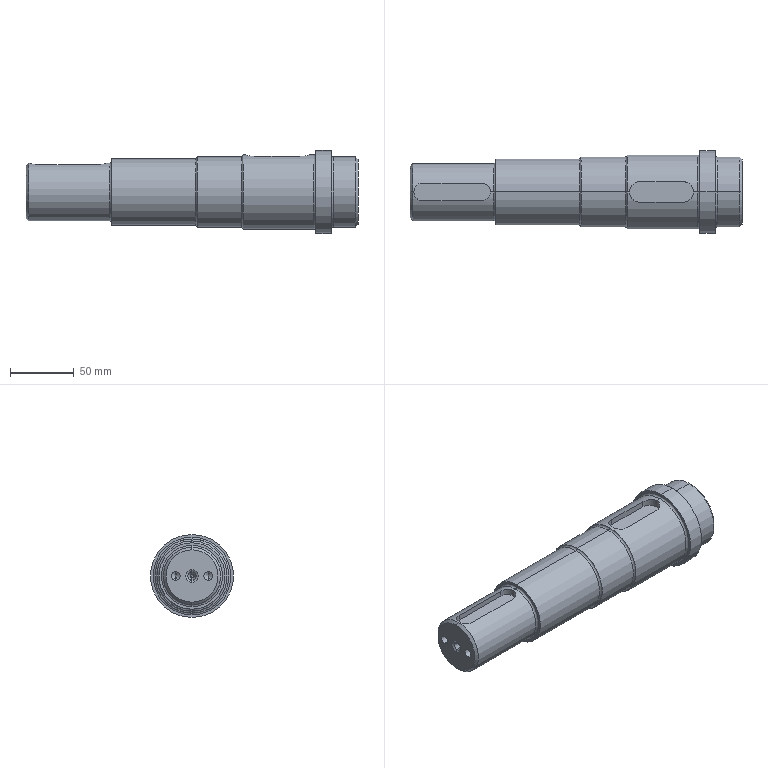Part | SolidWorks | features ICE 2, 3DProfileFeature 1, Chamfer 1, Fillet 1, HoleWzd 1, MirrorPattern 1, RevCut 1, Revolution 1 | 1 solid | 59 faces | box 260 x 65 x 65 mm | volume 565066 mm3 | cylinder 24 | cone 14 | plane 11 | torus 10 | commonest cylinder face diameters 6.8 x4 55 x4 14 x3 16 x3 3.15 x2 45 x2